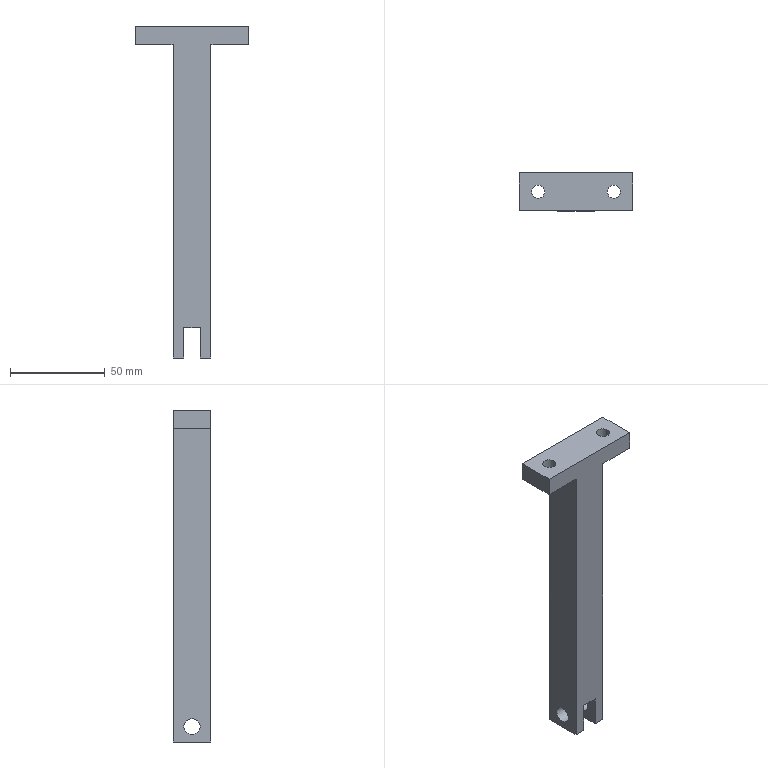Part | NX | features solid 2 | 1 solid | 19 faces | box 60 x 20 x 175 mm | volume 70289 mm3 | plane 15 | cylinder 4 | commonest cylinder face diameters 7 x2 8.5 x2
STEP:
#1=CARTESIAN_POINT('',(-695.,-480.,-105.));
#2=VERTEX_POINT('',#1);
#3=CARTESIAN_POINT('',(-689.25,-480.,-105.));
#4=VERTEX_POINT('',#3);
#5=CARTESIAN_POINT('',(-695.,-480.,-105.));
#6=DIRECTION('',(1.,0.,0.));
#7=VECTOR('',#6,1000.);
#8=LINE('',#5,#7);
#9=EDGE_CURVE('',#2,#4,#8,.T.);
#10=ORIENTED_EDGE('',*,*,#9,.F.);
#11=CARTESIAN_POINT('',(-695.,-460.,-105.));
#12=VERTEX_POINT('',#11);
#13=CARTESIAN_POINT('',(-695.,-460.,-105.));
#14=DIRECTION('',(0.,-1.,0.));
#15=VECTOR('',#14,1000.);
#16=LINE('',#13,#15);
#17=EDGE_CURVE('',#12,#2,#16,.T.);
#18=ORIENTED_EDGE('',*,*,#17,.F.);
#19=CARTESIAN_POINT('',(-689.25,-460.,-105.));
#20=VERTEX_POINT('',#19);
#21=CARTESIAN_POINT('',(-675.,-460.,-105.));
#22=DIRECTION('',(-1.,0.,0.));
#23=VECTOR('',#22,1000.);
#24=LINE('',#21,#23);
#25=EDGE_CURVE('',#20,#12,#24,.T.);
#26=ORIENTED_EDGE('',*,*,#25,.F.);
#27=CARTESIAN_POINT('',(-689.25,-460.,-105.));
#28=DIRECTION('',(0.,-1.,0.));
#29=VECTOR('',#28,1000.);
#30=LINE('',#27,#29);
#31=EDGE_CURVE('',#20,#4,#30,.T.);
#32=ORIENTED_EDGE('',*,*,#31,.T.);
#33=EDGE_LOOP('',(#10,#18,#26,#32));
#34=FACE_BOUND('',#33,.T.);
#35=CARTESIAN_POINT('',(-695.,-480.,-105.));
#36=DIRECTION('',(0.,0.,1.));
#37=DIRECTION('',(1.,0.,0.));
#38=AXIS2_PLACEMENT_3D('',#35,#36,#37);
#39=PLANE('',#38);
#40=ADVANCED_FACE('',(#34),#39,.F.);
#41=CARTESIAN_POINT('',(-675.,-480.,60.));
#42=VERTEX_POINT('',#41);
#43=CARTESIAN_POINT('',(-675.,-480.,-105.));
#44=VERTEX_POINT('',#43);
#45=CARTESIAN_POINT('',(-675.,-480.,55.));
#46=DIRECTION('',(0.,0.,-1.));
#47=VECTOR('',#46,1000.);
#48=LINE('',#45,#47);
#49=EDGE_CURVE('',#42,#44,#48,.T.);
#50=ORIENTED_EDGE('',*,*,#49,.F.);
#51=CARTESIAN_POINT('',(-655.,-480.,60.));
#52=VERTEX_POINT('',#51);
#53=CARTESIAN_POINT('',(-715.,-480.,60.));
#54=DIRECTION('',(1.,0.,0.));
#55=VECTOR('',#54,1000.);
#56=LINE('',#53,#55);
#57=EDGE_CURVE('',#42,#52,#56,.T.);
#58=ORIENTED_EDGE('',*,*,#57,.T.);
#59=CARTESIAN_POINT('',(-655.,-480.,70.));
#60=VERTEX_POINT('',#59);
#61=CARTESIAN_POINT('',(-655.,-480.,70.));
#62=DIRECTION('',(0.,0.,-1.));
#63=VECTOR('',#62,1000.);
#64=LINE('',#61,#63);
#65=EDGE_CURVE('',#60,#52,#64,.T.);
#66=ORIENTED_EDGE('',*,*,#65,.F.);
#67=CARTESIAN_POINT('',(-715.,-480.,70.));
#68=VERTEX_POINT('',#67);
#69=CARTESIAN_POINT('',(-695.,-480.,70.));
#70=DIRECTION('',(1.,0.,0.));
#71=VECTOR('',#70,1000.);
#72=LINE('',#69,#71);
#73=EDGE_CURVE('',#68,#60,#72,.T.);
#74=ORIENTED_EDGE('',*,*,#73,.F.);
#75=CARTESIAN_POINT('',(-715.,-480.,60.));
#76=VERTEX_POINT('',#75);
#77=CARTESIAN_POINT('',(-715.,-480.,70.));
#78=DIRECTION('',(0.,0.,-1.));
#79=VECTOR('',#78,1000.);
#80=LINE('',#77,#79);
#81=EDGE_CURVE('',#68,#76,#80,.T.);
#82=ORIENTED_EDGE('',*,*,#81,.T.);
#83=CARTESIAN_POINT('',(-695.,-480.,60.));
#84=VERTEX_POINT('',#83);
#85=CARTESIAN_POINT('',(-715.,-480.,60.));
#86=DIRECTION('',(1.,0.,0.));
#87=VECTOR('',#86,1000.);
#88=LINE('',#85,#87);
#89=EDGE_CURVE('',#76,#84,#88,.T.);
#90=ORIENTED_EDGE('',*,*,#89,.T.);
#91=CARTESIAN_POINT('',(-695.,-480.,55.));
#92=DIRECTION('',(0.,0.,-1.));
#93=VECTOR('',#92,1000.);
#94=LINE('',#91,#93);
#95=EDGE_CURVE('',#84,#2,#94,.T.);
#96=ORIENTED_EDGE('',*,*,#95,.T.);
#97=ORIENTED_EDGE('',*,*,#9,.T.);
#98=CARTESIAN_POINT('',(-689.25,-480.,-89.));
#99=VERTEX_POINT('',#98);
#100=CARTESIAN_POINT('',(-689.25,-480.,-89.));
#101=DIRECTION('',(0.,0.,-1.));
#102=VECTOR('',#101,1000.);
#103=LINE('',#100,#102);
#104=EDGE_CURVE('',#99,#4,#103,.T.);
#105=ORIENTED_EDGE('',*,*,#104,.F.);
#106=CARTESIAN_POINT('',(-680.75,-480.,-89.));
#107=VERTEX_POINT('',#106);
#108=CARTESIAN_POINT('',(-689.25,-480.,-89.));
#109=DIRECTION('',(1.,0.,0.));
#110=VECTOR('',#109,1000.);
#111=LINE('',#108,#110);
#112=EDGE_CURVE('',#99,#107,#111,.T.);
#113=ORIENTED_EDGE('',*,*,#112,.T.);
#114=CARTESIAN_POINT('',(-680.75,-480.,-105.));
#115=VERTEX_POINT('',#114);
#116=CARTESIAN_POINT('',(-680.75,-480.,-89.));
#117=DIRECTION('',(0.,0.,-1.));
#118=VECTOR('',#117,1000.);
#119=LINE('',#116,#118);
#120=EDGE_CURVE('',#107,#115,#119,.T.);
#121=ORIENTED_EDGE('',*,*,#120,.T.);
#122=CARTESIAN_POINT('',(-695.,-480.,-105.));
#123=DIRECTION('',(1.,0.,0.));
#124=VECTOR('',#123,1000.);
#125=LINE('',#122,#124);
#126=EDGE_CURVE('',#115,#44,#125,.T.);
#127=ORIENTED_EDGE('',*,*,#126,.T.);
#128=EDGE_LOOP('',(#50,#58,#66,#74,#82,#90,#96,#97,#105,#113,#121,#127));
#129=FACE_BOUND('',#128,.T.);
#130=CARTESIAN_POINT('',(-695.,-480.,55.));
#131=DIRECTION('',(0.,-1.,0.));
#132=DIRECTION('',(0.,0.,1.));
#133=AXIS2_PLACEMENT_3D('',#130,#131,#132);
#134=PLANE('',#133);
#135=ADVANCED_FACE('',(#129),#134,.T.);
#136=CARTESIAN_POINT('',(-675.,-474.25,-97.));
#137=VERTEX_POINT('',#136);
#138=CARTESIAN_POINT('',(-675.,-470.,-97.));
#139=DIRECTION('',(-1.,0.,0.));
#140=DIRECTION('',(0.,-1.,0.));
#141=AXIS2_PLACEMENT_3D('',#138,#139,#140);
#142=CIRCLE('',#141,4.25);
#143=EDGE_CURVE('',#137,#137,#142,.T.);
#144=ORIENTED_EDGE('',*,*,#143,.T.);
#145=EDGE_LOOP('',(#144));
#146=FACE_BOUND('',#145,.T.);
#147=CARTESIAN_POINT('',(-675.,-460.,60.));
#148=VERTEX_POINT('',#147);
#149=CARTESIAN_POINT('',(-675.,-480.,60.));
#150=DIRECTION('',(0.,-1.,0.));
#151=VECTOR('',#150,1000.);
#152=LINE('',#149,#151);
#153=EDGE_CURVE('',#148,#42,#152,.T.);
#154=ORIENTED_EDGE('',*,*,#153,.T.);
#155=ORIENTED_EDGE('',*,*,#49,.T.);
#156=CARTESIAN_POINT('',(-675.,-460.,-105.));
#157=VERTEX_POINT('',#156);
#158=CARTESIAN_POINT('',(-675.,-480.,-105.));
#159=DIRECTION('',(0.,1.,0.));
#160=VECTOR('',#159,1000.);
#161=LINE('',#158,#160);
#162=EDGE_CURVE('',#44,#157,#161,.T.);
#163=ORIENTED_EDGE('',*,*,#162,.T.);
#164=CARTESIAN_POINT('',(-675.,-460.,55.));
#165=DIRECTION('',(0.,0.,-1.));
#166=VECTOR('',#165,1000.);
#167=LINE('',#164,#166);
#168=EDGE_CURVE('',#148,#157,#167,.T.);
#169=ORIENTED_EDGE('',*,*,#168,.F.);
#170=EDGE_LOOP('',(#154,#155,#163,#169));
#171=FACE_BOUND('',#170,.T.);
#172=CARTESIAN_POINT('',(-675.,-480.,55.));
#173=DIRECTION('',(1.,0.,0.));
#174=DIRECTION('',(0.,-1.,0.));
#175=AXIS2_PLACEMENT_3D('',#172,#173,#174);
#176=PLANE('',#175);
#177=ADVANCED_FACE('',(#146,#171),#176,.T.);
#178=CARTESIAN_POINT('',(-695.,-460.,60.));
#179=VERTEX_POINT('',#178);
#180=CARTESIAN_POINT('',(-695.,-460.,55.));
#181=DIRECTION('',(0.,0.,-1.));
#182=VECTOR('',#181,1000.);
#183=LINE('',#180,#182);
#184=EDGE_CURVE('',#179,#12,#183,.T.);
#185=ORIENTED_EDGE('',*,*,#184,.F.);
#186=CARTESIAN_POINT('',(-715.,-460.,60.));
#187=VERTEX_POINT('',#186);
#188=CARTESIAN_POINT('',(-655.,-460.,60.));
#189=DIRECTION('',(-1.,0.,0.));
#190=VECTOR('',#189,1000.);
#191=LINE('',#188,#190);
#192=EDGE_CURVE('',#179,#187,#191,.T.);
#193=ORIENTED_EDGE('',*,*,#192,.T.);
#194=CARTESIAN_POINT('',(-715.,-460.,70.));
#195=VERTEX_POINT('',#194);
#196=CARTESIAN_POINT('',(-715.,-460.,70.));
#197=DIRECTION('',(0.,0.,-1.));
#198=VECTOR('',#197,1000.);
#199=LINE('',#196,#198);
#200=EDGE_CURVE('',#195,#187,#199,.T.);
#201=ORIENTED_EDGE('',*,*,#200,.F.);
#202=CARTESIAN_POINT('',(-655.,-460.,70.));
#203=VERTEX_POINT('',#202);
#204=CARTESIAN_POINT('',(-675.,-460.,70.));
#205=DIRECTION('',(-1.,0.,0.));
#206=VECTOR('',#205,1000.);
#207=LINE('',#204,#206);
#208=EDGE_CURVE('',#203,#195,#207,.T.);
#209=ORIENTED_EDGE('',*,*,#208,.F.);
#210=CARTESIAN_POINT('',(-655.,-460.,60.));
#211=VERTEX_POINT('',#210);
#212=CARTESIAN_POINT('',(-655.,-460.,70.));
#213=DIRECTION('',(0.,0.,-1.));
#214=VECTOR('',#213,1000.);
#215=LINE('',#212,#214);
#216=EDGE_CURVE('',#203,#211,#215,.T.);
#217=ORIENTED_EDGE('',*,*,#216,.T.);
#218=CARTESIAN_POINT('',(-655.,-460.,60.));
#219=DIRECTION('',(-1.,0.,0.));
#220=VECTOR('',#219,1000.);
#221=LINE('',#218,#220);
#222=EDGE_CURVE('',#211,#148,#221,.T.);
#223=ORIENTED_EDGE('',*,*,#222,.T.);
#224=ORIENTED_EDGE('',*,*,#168,.T.);
#225=CARTESIAN_POINT('',(-680.75,-460.,-105.));
#226=VERTEX_POINT('',#225);
#227=CARTESIAN_POINT('',(-675.,-460.,-105.));
#228=DIRECTION('',(-1.,0.,0.));
#229=VECTOR('',#228,1000.);
#230=LINE('',#227,#229);
#231=EDGE_CURVE('',#157,#226,#230,.T.);
#232=ORIENTED_EDGE('',*,*,#231,.T.);
#233=CARTESIAN_POINT('',(-680.75,-460.,-33.019));
#234=VERTEX_POINT('',#233);
#235=CARTESIAN_POINT('',(-680.75,-460.,-89.));
#236=DIRECTION('',(0.,0.,-1.));
#237=VECTOR('',#236,1000.);
#238=LINE('',#235,#237);
#239=EDGE_CURVE('',#234,#226,#238,.T.);
#240=ORIENTED_EDGE('',*,*,#239,.F.);
#241=CARTESIAN_POINT('',(-689.25,-460.,-33.019));
#242=VERTEX_POINT('',#241);
#243=CARTESIAN_POINT('',(-675.,-460.,-33.019));
#244=DIRECTION('',(1.,0.,0.));
#245=VECTOR('',#244,1000.);
#246=LINE('',#243,#245);
#247=EDGE_CURVE('',#242,#234,#246,.T.);
#248=ORIENTED_EDGE('',*,*,#247,.F.);
#249=CARTESIAN_POINT('',(-689.25,-460.,-89.));
#250=DIRECTION('',(0.,0.,-1.));
#251=VECTOR('',#250,1000.);
#252=LINE('',#249,#251);
#253=EDGE_CURVE('',#242,#20,#252,.T.);
#254=ORIENTED_EDGE('',*,*,#253,.T.);
#255=ORIENTED_EDGE('',*,*,#25,.T.);
#256=EDGE_LOOP('',(#185,#193,#201,#209,#217,#223,#224,#232,#240,#248,#254,#255));
#257=FACE_BOUND('',#256,.T.);
#258=CARTESIAN_POINT('',(-675.,-460.,55.));
#259=DIRECTION('',(0.,1.,0.));
#260=DIRECTION('',(1.,0.,0.));
#261=AXIS2_PLACEMENT_3D('',#258,#259,#260);
#262=PLANE('',#261);
#263=ADVANCED_FACE('',(#257),#262,.T.);
#264=CARTESIAN_POINT('',(-695.,-470.,-101.25));
#265=VERTEX_POINT('',#264);
#266=CARTESIAN_POINT('',(-695.,-470.,-97.));
#267=DIRECTION('',(-1.,0.,0.));
#268=DIRECTION('',(0.,0.,-1.));
#269=AXIS2_PLACEMENT_3D('',#266,#267,#268);
#270=CIRCLE('',#269,4.25);
#271=EDGE_CURVE('',#265,#265,#270,.T.);
#272=ORIENTED_EDGE('',*,*,#271,.F.);
#273=EDGE_LOOP('',(#272));
#274=FACE_BOUND('',#273,.T.);
#275=CARTESIAN_POINT('',(-695.,-480.,60.));
#276=DIRECTION('',(0.,1.,0.));
#277=VECTOR('',#276,1000.);
#278=LINE('',#275,#277);
#279=EDGE_CURVE('',#84,#179,#278,.T.);
#280=ORIENTED_EDGE('',*,*,#279,.T.);
#281=ORIENTED_EDGE('',*,*,#184,.T.);
#282=ORIENTED_EDGE('',*,*,#17,.T.);
#283=ORIENTED_EDGE('',*,*,#95,.F.);
#284=EDGE_LOOP('',(#280,#281,#282,#283));
#285=FACE_BOUND('',#284,.T.);
#286=CARTESIAN_POINT('',(-695.,-460.,55.));
#287=DIRECTION('',(-1.,0.,0.));
#288=DIRECTION('',(0.,0.,1.));
#289=AXIS2_PLACEMENT_3D('',#286,#287,#288);
#290=PLANE('',#289);
#291=ADVANCED_FACE('',(#274,#285),#290,.T.);
#292=ORIENTED_EDGE('',*,*,#231,.F.);
#293=ORIENTED_EDGE('',*,*,#162,.F.);
#294=ORIENTED_EDGE('',*,*,#126,.F.);
#295=CARTESIAN_POINT('',(-680.75,-480.,-105.));
#296=DIRECTION('',(0.,1.,0.));
#297=VECTOR('',#296,1000.);
#298=LINE('',#295,#297);
#299=EDGE_CURVE('',#115,#226,#298,.T.);
#300=ORIENTED_EDGE('',*,*,#299,.T.);
#301=EDGE_LOOP('',(#292,#293,#294,#300));
#302=FACE_BOUND('',#301,.T.);
#303=CARTESIAN_POINT('',(-695.,-480.,-105.));
#304=DIRECTION('',(0.,0.,1.));
#305=DIRECTION('',(1.,0.,0.));
#306=AXIS2_PLACEMENT_3D('',#303,#304,#305);
#307=PLANE('',#306);
#308=ADVANCED_FACE('',(#302),#307,.F.);
#309=CARTESIAN_POINT('',(-689.25,-470.,-92.75));
#310=VERTEX_POINT('',#309);
#311=CARTESIAN_POINT('',(-689.25,-470.,-97.));
#312=DIRECTION('',(1.,0.,0.));
#313=DIRECTION('',(0.,0.,1.));
#314=AXIS2_PLACEMENT_3D('',#311,#312,#313);
#315=CIRCLE('',#314,4.25);
#316=EDGE_CURVE('',#310,#310,#315,.T.);
#317=ORIENTED_EDGE('',*,*,#316,.F.);
#318=EDGE_LOOP('',(#317));
#319=FACE_BOUND('',#318,.T.);
#320=ORIENTED_EDGE('',*,*,#31,.F.);
#321=ORIENTED_EDGE('',*,*,#253,.F.);
#322=CARTESIAN_POINT('',(-689.25,-475.,-89.));
#323=VERTEX_POINT('',#322);
#324=CARTESIAN_POINT('',(-689.25,-473.995,-85.25));
#325=DIRECTION('',(0.,-0.2588,-0.9659));
#326=VECTOR('',#325,1000.);
#327=LINE('',#324,#326);
#328=EDGE_CURVE('',#323,#242,#327,.F.);
#329=ORIENTED_EDGE('',*,*,#328,.F.);
#330=CARTESIAN_POINT('',(-689.25,-460.,-89.));
#331=DIRECTION('',(0.,-1.,0.));
#332=VECTOR('',#331,1000.);
#333=LINE('',#330,#332);
#334=EDGE_CURVE('',#323,#99,#333,.T.);
#335=ORIENTED_EDGE('',*,*,#334,.T.);
#336=ORIENTED_EDGE('',*,*,#104,.T.);
#337=EDGE_LOOP('',(#320,#321,#329,#335,#336));
#338=FACE_BOUND('',#337,.T.);
#339=CARTESIAN_POINT('',(-689.25,-460.,-89.));
#340=DIRECTION('',(-1.,0.,0.));
#341=DIRECTION('',(0.,0.,1.));
#342=AXIS2_PLACEMENT_3D('',#339,#340,#341);
#343=PLANE('',#342);
#344=ADVANCED_FACE('',(#319,#338),#343,.F.);
#345=CARTESIAN_POINT('',(-680.75,-474.25,-97.));
#346=VERTEX_POINT('',#345);
#347=CARTESIAN_POINT('',(-680.75,-470.,-97.));
#348=DIRECTION('',(-1.,0.,0.));
#349=DIRECTION('',(0.,-1.,0.));
#350=AXIS2_PLACEMENT_3D('',#347,#348,#349);
#351=CIRCLE('',#350,4.25);
#352=EDGE_CURVE('',#346,#346,#351,.T.);
#353=ORIENTED_EDGE('',*,*,#352,.F.);
#354=EDGE_LOOP('',(#353));
#355=FACE_BOUND('',#354,.T.);
#356=ORIENTED_EDGE('',*,*,#299,.F.);
#357=ORIENTED_EDGE('',*,*,#120,.F.);
#358=CARTESIAN_POINT('',(-680.75,-475.,-89.));
#359=VERTEX_POINT('',#358);
#360=CARTESIAN_POINT('',(-680.75,-480.,-89.));
#361=DIRECTION('',(0.,1.,0.));
#362=VECTOR('',#361,1000.);
#363=LINE('',#360,#362);
#364=EDGE_CURVE('',#107,#359,#363,.T.);
#365=ORIENTED_EDGE('',*,*,#364,.T.);
#366=CARTESIAN_POINT('',(-680.75,-475.335,-90.25));
#367=DIRECTION('',(0.,0.2588,0.9659));
#368=VECTOR('',#367,1000.);
#369=LINE('',#366,#368);
#370=EDGE_CURVE('',#234,#359,#369,.F.);
#371=ORIENTED_EDGE('',*,*,#370,.F.);
#372=ORIENTED_EDGE('',*,*,#239,.T.);
#373=EDGE_LOOP('',(#356,#357,#365,#371,#372));
#374=FACE_BOUND('',#373,.T.);
#375=CARTESIAN_POINT('',(-680.75,-480.,-89.));
#376=DIRECTION('',(1.,0.,0.));
#377=DIRECTION('',(0.,-1.,0.));
#378=AXIS2_PLACEMENT_3D('',#375,#376,#377);
#379=PLANE('',#378);
#380=ADVANCED_FACE('',(#355,#374),#379,.F.);
#381=ORIENTED_EDGE('',*,*,#364,.F.);
#382=ORIENTED_EDGE('',*,*,#112,.F.);
#383=ORIENTED_EDGE('',*,*,#334,.F.);
#384=CARTESIAN_POINT('',(-689.25,-475.,-89.));
#385=DIRECTION('',(-1.,0.,0.));
#386=VECTOR('',#385,1000.);
#387=LINE('',#384,#386);
#388=EDGE_CURVE('',#359,#323,#387,.T.);
#389=ORIENTED_EDGE('',*,*,#388,.F.);
#390=EDGE_LOOP('',(#381,#382,#383,#389));
#391=FACE_BOUND('',#390,.T.);
#392=CARTESIAN_POINT('',(-689.25,-460.,-89.));
#393=DIRECTION('',(0.,0.,-1.));
#394=DIRECTION('',(-1.,0.,0.));
#395=AXIS2_PLACEMENT_3D('',#392,#393,#394);
#396=PLANE('',#395);
#397=ADVANCED_FACE('',(#391),#396,.T.);
#398=ORIENTED_EDGE('',*,*,#370,.T.);
#399=ORIENTED_EDGE('',*,*,#388,.T.);
#400=ORIENTED_EDGE('',*,*,#328,.T.);
#401=ORIENTED_EDGE('',*,*,#247,.T.);
#402=EDGE_LOOP('',(#398,#399,#400,#401));
#403=FACE_BOUND('',#402,.T.);
#404=CARTESIAN_POINT('',(-689.25,-475.,-89.));
#405=DIRECTION('',(0.,-0.9659,0.2588));
#406=DIRECTION('',(0.,0.2588,0.9659));
#407=AXIS2_PLACEMENT_3D('',#404,#405,#406);
#408=PLANE('',#407);
#409=ADVANCED_FACE('',(#403),#408,.F.);
#410=ORIENTED_EDGE('',*,*,#143,.F.);
#411=EDGE_LOOP('',(#410));
#412=FACE_BOUND('',#411,.T.);
#413=ORIENTED_EDGE('',*,*,#352,.T.);
#414=EDGE_LOOP('',(#413));
#415=FACE_BOUND('',#414,.T.);
#416=CARTESIAN_POINT('',(-695.,-470.,-97.));
#417=DIRECTION('',(1.,0.,0.));
#418=DIRECTION('',(0.,0.,-1.));
#419=AXIS2_PLACEMENT_3D('',#416,#417,#418);
#420=CYLINDRICAL_SURFACE('',#419,4.25);
#421=ADVANCED_FACE('',(#412,#415),#420,.F.);
#422=ORIENTED_EDGE('',*,*,#271,.T.);
#423=EDGE_LOOP('',(#422));
#424=FACE_BOUND('',#423,.T.);
#425=ORIENTED_EDGE('',*,*,#316,.T.);
#426=EDGE_LOOP('',(#425));
#427=FACE_BOUND('',#426,.T.);
#428=CARTESIAN_POINT('',(-695.,-470.,-97.));
#429=DIRECTION('',(1.,0.,0.));
#430=DIRECTION('',(0.,0.,-1.));
#431=AXIS2_PLACEMENT_3D('',#428,#429,#430);
#432=CYLINDRICAL_SURFACE('',#431,4.25);
#433=ADVANCED_FACE('',(#424,#427),#432,.F.);
#434=CARTESIAN_POINT('',(-708.5,-470.,60.));
#435=VERTEX_POINT('',#434);
#436=CARTESIAN_POINT('',(-705.,-470.,60.));
#437=DIRECTION('',(0.,0.,1.));
#438=DIRECTION('',(-1.,0.,0.));
#439=AXIS2_PLACEMENT_3D('',#436,#437,#438);
#440=CIRCLE('',#439,3.5);
#441=EDGE_CURVE('',#435,#435,#440,.T.);
#442=ORIENTED_EDGE('',*,*,#441,.T.);
#443=EDGE_LOOP('',(#442));
#444=FACE_BOUND('',#443,.T.);
#445=ORIENTED_EDGE('',*,*,#279,.F.);
#446=ORIENTED_EDGE('',*,*,#89,.F.);
#447=CARTESIAN_POINT('',(-715.,-460.,60.));
#448=DIRECTION('',(0.,-1.,0.));
#449=VECTOR('',#448,1000.);
#450=LINE('',#447,#449);
#451=EDGE_CURVE('',#187,#76,#450,.T.);
#452=ORIENTED_EDGE('',*,*,#451,.F.);
#453=ORIENTED_EDGE('',*,*,#192,.F.);
#454=EDGE_LOOP('',(#445,#446,#452,#453));
#455=FACE_BOUND('',#454,.T.);
#456=CARTESIAN_POINT('',(-655.,-480.,60.));
#457=DIRECTION('',(0.,0.,-1.));
#458=DIRECTION('',(-1.,0.,0.));
#459=AXIS2_PLACEMENT_3D('',#456,#457,#458);
#460=PLANE('',#459);
#461=ADVANCED_FACE('',(#444,#455),#460,.T.);
#462=CARTESIAN_POINT('',(-668.5,-470.,60.));
#463=VERTEX_POINT('',#462);
#464=CARTESIAN_POINT('',(-665.,-470.,60.));
#465=DIRECTION('',(0.,0.,1.));
#466=DIRECTION('',(-1.,0.,0.));
#467=AXIS2_PLACEMENT_3D('',#464,#465,#466);
#468=CIRCLE('',#467,3.5);
#469=EDGE_CURVE('',#463,#463,#468,.T.);
#470=ORIENTED_EDGE('',*,*,#469,.T.);
#471=EDGE_LOOP('',(#470));
#472=FACE_BOUND('',#471,.T.);
#473=ORIENTED_EDGE('',*,*,#153,.F.);
#474=ORIENTED_EDGE('',*,*,#222,.F.);
#475=CARTESIAN_POINT('',(-655.,-480.,60.));
#476=DIRECTION('',(0.,1.,0.));
#477=VECTOR('',#476,1000.);
#478=LINE('',#475,#477);
#479=EDGE_CURVE('',#52,#211,#478,.T.);
#480=ORIENTED_EDGE('',*,*,#479,.F.);
#481=ORIENTED_EDGE('',*,*,#57,.F.);
#482=EDGE_LOOP('',(#473,#474,#480,#481));
#483=FACE_BOUND('',#482,.T.);
#484=CARTESIAN_POINT('',(-655.,-480.,60.));
#485=DIRECTION('',(0.,0.,-1.));
#486=DIRECTION('',(-1.,0.,0.));
#487=AXIS2_PLACEMENT_3D('',#484,#485,#486);
#488=PLANE('',#487);
#489=ADVANCED_FACE('',(#472,#483),#488,.T.);
#490=CARTESIAN_POINT('',(-708.5,-470.,70.));
#491=VERTEX_POINT('',#490);
#492=CARTESIAN_POINT('',(-705.,-470.,70.));
#493=DIRECTION('',(0.,0.,1.));
#494=DIRECTION('',(-1.,0.,0.));
#495=AXIS2_PLACEMENT_3D('',#492,#493,#494);
#496=CIRCLE('',#495,3.5);
#497=EDGE_CURVE('',#491,#491,#496,.T.);
#498=ORIENTED_EDGE('',*,*,#497,.F.);
#499=EDGE_LOOP('',(#498));
#500=FACE_BOUND('',#499,.T.);
#501=CARTESIAN_POINT('',(-668.5,-470.,70.));
#502=VERTEX_POINT('',#501);
#503=CARTESIAN_POINT('',(-665.,-470.,70.));
#504=DIRECTION('',(0.,0.,1.));
#505=DIRECTION('',(-1.,0.,0.));
#506=AXIS2_PLACEMENT_3D('',#503,#504,#505);
#507=CIRCLE('',#506,3.5);
#508=EDGE_CURVE('',#502,#502,#507,.T.);
#509=ORIENTED_EDGE('',*,*,#508,.F.);
#510=EDGE_LOOP('',(#509));
#511=FACE_BOUND('',#510,.T.);
#512=ORIENTED_EDGE('',*,*,#73,.T.);
#513=CARTESIAN_POINT('',(-655.,-480.,70.));
#514=DIRECTION('',(0.,1.,0.));
#515=VECTOR('',#514,1000.);
#516=LINE('',#513,#515);
#517=EDGE_CURVE('',#60,#203,#516,.T.);
#518=ORIENTED_EDGE('',*,*,#517,.T.);
#519=ORIENTED_EDGE('',*,*,#208,.T.);
#520=CARTESIAN_POINT('',(-715.,-460.,70.));
#521=DIRECTION('',(0.,-1.,0.));
#522=VECTOR('',#521,1000.);
#523=LINE('',#520,#522);
#524=EDGE_CURVE('',#195,#68,#523,.T.);
#525=ORIENTED_EDGE('',*,*,#524,.T.);
#526=EDGE_LOOP('',(#512,#518,#519,#525));
#527=FACE_BOUND('',#526,.T.);
#528=CARTESIAN_POINT('',(-695.,-480.,70.));
#529=DIRECTION('',(0.,0.,1.));
#530=DIRECTION('',(1.,0.,0.));
#531=AXIS2_PLACEMENT_3D('',#528,#529,#530);
#532=PLANE('',#531);
#533=ADVANCED_FACE('',(#500,#511,#527),#532,.T.);
#534=ORIENTED_EDGE('',*,*,#451,.T.);
#535=ORIENTED_EDGE('',*,*,#81,.F.);
#536=ORIENTED_EDGE('',*,*,#524,.F.);
#537=ORIENTED_EDGE('',*,*,#200,.T.);
#538=EDGE_LOOP('',(#534,#535,#536,#537));
#539=FACE_BOUND('',#538,.T.);
#540=CARTESIAN_POINT('',(-715.,-460.,70.));
#541=DIRECTION('',(-1.,0.,0.));
#542=DIRECTION('',(0.,0.,1.));
#543=AXIS2_PLACEMENT_3D('',#540,#541,#542);
#544=PLANE('',#543);
#545=ADVANCED_FACE('',(#539),#544,.T.);
#546=ORIENTED_EDGE('',*,*,#441,.F.);
#547=EDGE_LOOP('',(#546));
#548=FACE_BOUND('',#547,.T.);
#549=ORIENTED_EDGE('',*,*,#497,.T.);
#550=EDGE_LOOP('',(#549));
#551=FACE_BOUND('',#550,.T.);
#552=CARTESIAN_POINT('',(-705.,-470.,70.));
#553=DIRECTION('',(0.,0.,-1.));
#554=DIRECTION('',(-1.,0.,0.));
#555=AXIS2_PLACEMENT_3D('',#552,#553,#554);
#556=CYLINDRICAL_SURFACE('',#555,3.5);
#557=ADVANCED_FACE('',(#548,#551),#556,.F.);
#558=ORIENTED_EDGE('',*,*,#479,.T.);
#559=ORIENTED_EDGE('',*,*,#216,.F.);
#560=ORIENTED_EDGE('',*,*,#517,.F.);
#561=ORIENTED_EDGE('',*,*,#65,.T.);
#562=EDGE_LOOP('',(#558,#559,#560,#561));
#563=FACE_BOUND('',#562,.T.);
#564=CARTESIAN_POINT('',(-655.,-480.,70.));
#565=DIRECTION('',(1.,0.,0.));
#566=DIRECTION('',(0.,0.,-1.));
#567=AXIS2_PLACEMENT_3D('',#564,#565,#566);
#568=PLANE('',#567);
#569=ADVANCED_FACE('',(#563),#568,.T.);
#570=ORIENTED_EDGE('',*,*,#469,.F.);
#571=EDGE_LOOP('',(#570));
#572=FACE_BOUND('',#571,.T.);
#573=ORIENTED_EDGE('',*,*,#508,.T.);
#574=EDGE_LOOP('',(#573));
#575=FACE_BOUND('',#574,.T.);
#576=CARTESIAN_POINT('',(-665.,-470.,70.));
#577=DIRECTION('',(0.,0.,-1.));
#578=DIRECTION('',(-1.,0.,0.));
#579=AXIS2_PLACEMENT_3D('',#576,#577,#578);
#580=CYLINDRICAL_SURFACE('',#579,3.5);
#581=ADVANCED_FACE('',(#572,#575),#580,.F.);
#582=CLOSED_SHELL('',(#40,#135,#177,#263,#291,#308,#344,#380,#397,#409,#421,#433,#461,#489,#533,#545,#557,#569,#581));
#583=MANIFOLD_SOLID_BREP('',#582);
#584=(LENGTH_UNIT()NAMED_UNIT(*)SI_UNIT(.MILLI.,.METRE.));
#585=UNCERTAINTY_MEASURE_WITH_UNIT(LENGTH_MEASURE(0.00001),#584,'','');
#586=(NAMED_UNIT(*)PLANE_ANGLE_UNIT()SI_UNIT($,.RADIAN.));
#587=(NAMED_UNIT(*)SI_UNIT($,.STERADIAN.)SOLID_ANGLE_UNIT());
#588=(GEOMETRIC_REPRESENTATION_CONTEXT(3)GLOBAL_UNCERTAINTY_ASSIGNED_CONTEXT((#585))GLOBAL_UNIT_ASSIGNED_CONTEXT((#584,#586,#587))REPRESENTATION_CONTEXT('',''));
#589=ADVANCED_BREP_SHAPE_REPRESENTATION('',(#583),#588);